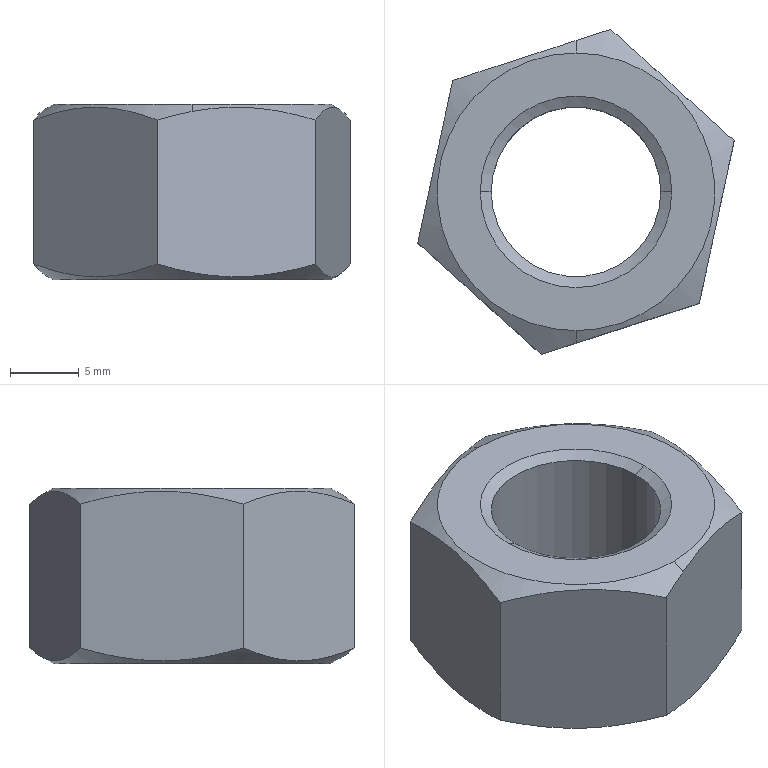Part | SolidWorks | features BaseBody 1 | 1 solid | 18 faces | box 23.075 x 23.71 x 12.8 mm | volume 3293 mm3 | cone 8 | plane 8 | cylinder 2 | commonest cylinder face diameters 12.376 x2
STEP:
#1=CARTESIAN_POINT('',(228.812,0.,355.481));
#2=VERTEX_POINT('',#1);
#3=CARTESIAN_POINT('',(241.188,0.,355.481));
#4=VERTEX_POINT('',#3);
#5=CARTESIAN_POINT('',(235.,0.,355.481));
#6=DIRECTION('',(0.,0.,1.));
#7=DIRECTION('',(1.,0.,0.));
#8=AXIS2_PLACEMENT_3D('',#5,#6,#7);
#9=CIRCLE('',#8,6.188);
#10=EDGE_CURVE('',#2,#4,#9,.T.);
#11=ORIENTED_EDGE('',*,*,#10,.F.);
#12=CARTESIAN_POINT('',(228.812,0.,367.019));
#13=VERTEX_POINT('',#12);
#14=CARTESIAN_POINT('',(228.812,0.,354.681));
#15=DIRECTION('',(0.,0.,1.));
#16=VECTOR('',#15,1000.);
#17=LINE('',#14,#16);
#18=EDGE_CURVE('',#2,#13,#17,.T.);
#19=ORIENTED_EDGE('',*,*,#18,.T.);
#20=CARTESIAN_POINT('',(241.188,0.,367.019));
#21=VERTEX_POINT('',#20);
#22=CARTESIAN_POINT('',(235.,0.,367.019));
#23=DIRECTION('',(0.,0.,-1.));
#24=DIRECTION('',(1.,0.,0.));
#25=AXIS2_PLACEMENT_3D('',#22,#23,#24);
#26=CIRCLE('',#25,6.188);
#27=EDGE_CURVE('',#21,#13,#26,.T.);
#28=ORIENTED_EDGE('',*,*,#27,.F.);
#29=CARTESIAN_POINT('',(241.188,0.,354.681));
#30=DIRECTION('',(0.,0.,1.));
#31=VECTOR('',#30,1000.);
#32=LINE('',#29,#31);
#33=EDGE_CURVE('',#4,#21,#32,.T.);
#34=ORIENTED_EDGE('',*,*,#33,.F.);
#35=EDGE_LOOP('',(#11,#19,#28,#34));
#36=FACE_OUTER_BOUND('',#35,.T.);
#37=CARTESIAN_POINT('',(235.,0.,354.681));
#38=DIRECTION('',(0.,0.,1.));
#39=DIRECTION('',(1.,0.,0.));
#40=AXIS2_PLACEMENT_3D('',#37,#38,#39);
#41=CYLINDRICAL_SURFACE('',#40,6.188);
#42=ADVANCED_FACE('',(#36),#41,.F.);
#43=ORIENTED_EDGE('',*,*,#27,.T.);
#44=CARTESIAN_POINT('',(228.012,0.,367.481));
#45=VERTEX_POINT('',#44);
#46=CARTESIAN_POINT('',(228.012,0.,367.481));
#47=DIRECTION('',(-0.866,0.,0.5));
#48=VECTOR('',#47,1000.);
#49=LINE('',#46,#48);
#50=EDGE_CURVE('',#13,#45,#49,.T.);
#51=ORIENTED_EDGE('',*,*,#50,.T.);
#52=CARTESIAN_POINT('',(241.988,0.,367.481));
#53=VERTEX_POINT('',#52);
#54=CARTESIAN_POINT('',(235.,0.,367.481));
#55=DIRECTION('',(0.,0.,-1.));
#56=DIRECTION('',(1.,0.,0.));
#57=AXIS2_PLACEMENT_3D('',#54,#55,#56);
#58=CIRCLE('',#57,6.988);
#59=EDGE_CURVE('',#53,#45,#58,.T.);
#60=ORIENTED_EDGE('',*,*,#59,.F.);
#61=CARTESIAN_POINT('',(241.988,0.,367.481));
#62=DIRECTION('',(0.866,0.,0.5));
#63=VECTOR('',#62,1000.);
#64=LINE('',#61,#63);
#65=EDGE_CURVE('',#21,#53,#64,.T.);
#66=ORIENTED_EDGE('',*,*,#65,.F.);
#67=EDGE_LOOP('',(#43,#51,#60,#66));
#68=FACE_OUTER_BOUND('',#67,.T.);
#69=CARTESIAN_POINT('',(235.,0.,367.481));
#70=DIRECTION('',(0.,0.,1.));
#71=DIRECTION('',(1.,0.,0.));
#72=AXIS2_PLACEMENT_3D('',#69,#70,#71);
#73=CONICAL_SURFACE('',#72,6.988,1.047);
#74=ADVANCED_FACE('',(#68),#73,.F.);
#75=ORIENTED_EDGE('',*,*,#10,.T.);
#76=CARTESIAN_POINT('',(241.65,0.,354.681));
#77=VERTEX_POINT('',#76);
#78=CARTESIAN_POINT('',(241.65,0.,354.681));
#79=DIRECTION('',(0.5,0.,-0.866));
#80=VECTOR('',#79,1000.);
#81=LINE('',#78,#80);
#82=EDGE_CURVE('',#4,#77,#81,.T.);
#83=ORIENTED_EDGE('',*,*,#82,.T.);
#84=CARTESIAN_POINT('',(228.35,0.,354.681));
#85=VERTEX_POINT('',#84);
#86=CARTESIAN_POINT('',(235.,0.,354.681));
#87=DIRECTION('',(0.,0.,1.));
#88=DIRECTION('',(-1.,0.,0.));
#89=AXIS2_PLACEMENT_3D('',#86,#87,#88);
#90=CIRCLE('',#89,6.65);
#91=EDGE_CURVE('',#85,#77,#90,.T.);
#92=ORIENTED_EDGE('',*,*,#91,.F.);
#93=CARTESIAN_POINT('',(228.35,0.,354.681));
#94=DIRECTION('',(-0.5,0.,-0.866));
#95=VECTOR('',#94,1000.);
#96=LINE('',#93,#95);
#97=EDGE_CURVE('',#2,#85,#96,.T.);
#98=ORIENTED_EDGE('',*,*,#97,.F.);
#99=EDGE_LOOP('',(#75,#83,#92,#98));
#100=FACE_OUTER_BOUND('',#99,.T.);
#101=CARTESIAN_POINT('',(235.,0.,354.681));
#102=DIRECTION('',(0.,0.,-1.));
#103=DIRECTION('',(-1.,0.,0.));
#104=AXIS2_PLACEMENT_3D('',#101,#102,#103);
#105=CONICAL_SURFACE('',#104,6.65,0.5236);
#106=ADVANCED_FACE('',(#100),#105,.F.);
#107=CARTESIAN_POINT('',(235.,-10.125,367.481));
#108=VERTEX_POINT('',#107);
#109=CARTESIAN_POINT('',(235.,10.125,367.481));
#110=VERTEX_POINT('',#109);
#111=CARTESIAN_POINT('',(235.,0.,367.481));
#112=DIRECTION('',(0.,0.,1.));
#113=DIRECTION('',(0.,1.,0.));
#114=AXIS2_PLACEMENT_3D('',#111,#112,#113);
#115=CIRCLE('',#114,10.125);
#116=EDGE_CURVE('',#108,#110,#115,.T.);
#117=ORIENTED_EDGE('',*,*,#116,.F.);
#118=CARTESIAN_POINT('',(235.,-11.034,366.956));
#119=VERTEX_POINT('',#118);
#120=CARTESIAN_POINT('',(235.,-12.136,366.32));
#121=DIRECTION('',(0.,-0.866,-0.5));
#122=VECTOR('',#121,1000.);
#123=LINE('',#120,#122);
#124=EDGE_CURVE('',#108,#119,#123,.T.);
#125=ORIENTED_EDGE('',*,*,#124,.T.);
#126=CARTESIAN_POINT('',(243.995,-8.129,366.327));
#127=VERTEX_POINT('',#126);
#128=CARTESIAN_POINT('',(235.,-11.034,366.956));
#129=CARTESIAN_POINT('',(235.743,-10.794,367.095));
#130=CARTESIAN_POINT('',(236.492,-10.552,367.191));
#131=CARTESIAN_POINT('',(237.626,-10.186,367.258));
#132=CARTESIAN_POINT('',(238.005,-10.063,367.267));
#133=CARTESIAN_POINT('',(238.768,-9.817,367.26));
#134=CARTESIAN_POINT('',(239.151,-9.694,367.243));
#135=CARTESIAN_POINT('',(241.046,-9.082,367.094));
#136=CARTESIAN_POINT('',(242.53,-8.602,366.771));
#137=CARTESIAN_POINT('',(243.995,-8.129,366.327));
#138=B_SPLINE_CURVE_WITH_KNOTS('',3,(#128,#129,#130,#131,#132,#133,#134,#135,#136,#137),.UNSPECIFIED.,.F.,.F.,(4,2,2,2,4),(0.002734,0.005112,0.006301,0.007489,0.01224),.UNSPECIFIED.);
#139=EDGE_CURVE('',#119,#127,#138,.T.);
#140=ORIENTED_EDGE('',*,*,#139,.T.);
#141=CARTESIAN_POINT('',(246.538,3.726,366.327));
#142=VERTEX_POINT('',#141);
#143=CARTESIAN_POINT('',(243.995,-8.129,366.327));
#144=CARTESIAN_POINT('',(244.203,-7.161,366.612));
#145=CARTESIAN_POINT('',(244.412,-6.186,366.848));
#146=CARTESIAN_POINT('',(244.835,-4.216,367.174));
#147=CARTESIAN_POINT('',(245.048,-3.221,367.264));
#148=CARTESIAN_POINT('',(245.372,-1.709,367.265));
#149=CARTESIAN_POINT('',(245.481,-1.203,367.243));
#150=CARTESIAN_POINT('',(245.696,-0.2013,367.157));
#151=CARTESIAN_POINT('',(245.802,0.2961,367.094));
#152=CARTESIAN_POINT('',(246.12,1.779,366.849));
#153=CARTESIAN_POINT('',(246.33,2.757,366.613));
#154=CARTESIAN_POINT('',(246.538,3.726,366.327));
#155=B_SPLINE_CURVE_WITH_KNOTS('',3,(#143,#144,#145,#146,#147,#148,#149,#150,#151,#152,#153,#154),.UNSPECIFIED.,.F.,.F.,(4,2,2,2,2,4),(0.,0.003061,0.006122,0.007653,0.009184,0.01224),.UNSPECIFIED.);
#156=EDGE_CURVE('',#127,#142,#155,.T.);
#157=ORIENTED_EDGE('',*,*,#156,.T.);
#158=CARTESIAN_POINT('',(237.542,11.855,366.327));
#159=VERTEX_POINT('',#158);
#160=CARTESIAN_POINT('',(246.538,3.726,366.327));
#161=CARTESIAN_POINT('',(245.803,4.39,366.613));
#162=CARTESIAN_POINT('',(245.062,5.059,366.848));
#163=CARTESIAN_POINT('',(243.565,6.412,367.175));
#164=CARTESIAN_POINT('',(242.808,7.097,367.265));
#165=CARTESIAN_POINT('',(241.272,8.484,367.265));
#166=CARTESIAN_POINT('',(240.515,9.168,367.175));
#167=CARTESIAN_POINT('',(239.018,10.522,366.848));
#168=CARTESIAN_POINT('',(238.277,11.191,366.613));
#169=CARTESIAN_POINT('',(237.542,11.855,366.327));
#170=B_SPLINE_CURVE_WITH_KNOTS('',3,(#160,#161,#162,#163,#164,#165,#166,#167,#168,#169),.UNSPECIFIED.,.F.,.F.,(4,2,2,2,4),(0.,0.003067,0.006134,0.009201,0.01227),.UNSPECIFIED.);
#171=EDGE_CURVE('',#142,#159,#170,.T.);
#172=ORIENTED_EDGE('',*,*,#171,.T.);
#173=CARTESIAN_POINT('',(235.,11.034,366.956));
#174=VERTEX_POINT('',#173);
#175=CARTESIAN_POINT('',(237.542,11.855,366.327));
#176=CARTESIAN_POINT('',(236.701,11.583,366.582));
#177=CARTESIAN_POINT('',(235.854,11.31,366.797));
#178=CARTESIAN_POINT('',(235.,11.034,366.956));
#179=B_SPLINE_CURVE_WITH_KNOTS('',3,(#175,#176,#177,#178),.UNSPECIFIED.,.F.,.F.,(4,4),(0.,0.002734),.UNSPECIFIED.);
#180=EDGE_CURVE('',#159,#174,#179,.T.);
#181=ORIENTED_EDGE('',*,*,#180,.T.);
#182=CARTESIAN_POINT('',(235.,12.136,366.32));
#183=DIRECTION('',(0.,0.866,-0.5));
#184=VECTOR('',#183,1000.);
#185=LINE('',#182,#184);
#186=EDGE_CURVE('',#110,#174,#185,.T.);
#187=ORIENTED_EDGE('',*,*,#186,.F.);
#188=EDGE_LOOP('',(#117,#125,#140,#157,#172,#181,#187));
#189=FACE_OUTER_BOUND('',#188,.T.);
#190=CARTESIAN_POINT('',(235.,0.,366.32));
#191=DIRECTION('',(0.,0.,-1.));
#192=DIRECTION('',(0.,1.,0.));
#193=AXIS2_PLACEMENT_3D('',#190,#191,#192);
#194=CONICAL_SURFACE('',#193,12.136,1.047);
#195=ADVANCED_FACE('',(#189),#194,.T.);
#196=CARTESIAN_POINT('',(245.125,0.,354.681));
#197=VERTEX_POINT('',#196);
#198=CARTESIAN_POINT('',(224.875,0.,354.681));
#199=VERTEX_POINT('',#198);
#200=CARTESIAN_POINT('',(235.,0.,354.681));
#201=DIRECTION('',(0.,0.,1.));
#202=DIRECTION('',(1.,0.,0.));
#203=AXIS2_PLACEMENT_3D('',#200,#201,#202);
#204=CIRCLE('',#203,10.125);
#205=EDGE_CURVE('',#197,#199,#204,.T.);
#206=ORIENTED_EDGE('',*,*,#205,.T.);
#207=CARTESIAN_POINT('',(224.261,0.,355.035));
#208=VERTEX_POINT('',#207);
#209=CARTESIAN_POINT('',(222.864,0.,355.842));
#210=DIRECTION('',(-0.866,0.,0.5));
#211=VECTOR('',#210,1000.);
#212=LINE('',#209,#211);
#213=EDGE_CURVE('',#199,#208,#212,.T.);
#214=ORIENTED_EDGE('',*,*,#213,.T.);
#215=CARTESIAN_POINT('',(226.005,8.129,355.835));
#216=VERTEX_POINT('',#215);
#217=CARTESIAN_POINT('',(224.261,0.,355.035));
#218=CARTESIAN_POINT('',(224.406,0.6764,354.952));
#219=CARTESIAN_POINT('',(224.552,1.358,354.904));
#220=CARTESIAN_POINT('',(224.774,2.389,354.895));
#221=CARTESIAN_POINT('',(224.848,2.735,354.902));
#222=CARTESIAN_POINT('',(224.995,3.422,354.937));
#223=CARTESIAN_POINT('',(225.069,3.765,354.964));
#224=CARTESIAN_POINT('',(225.434,5.468,355.148));
#225=CARTESIAN_POINT('',(225.721,6.806,355.445));
#226=CARTESIAN_POINT('',(226.005,8.129,355.835));
#227=B_SPLINE_CURVE_WITH_KNOTS('',3,(#217,#218,#219,#220,#221,#222,#223,#224,#225,#226),.UNSPECIFIED.,.F.,.F.,(4,2,2,2,4),(0.003885,0.005975,0.00702,0.008065,0.01224),.UNSPECIFIED.);
#228=EDGE_CURVE('',#208,#216,#227,.T.);
#229=ORIENTED_EDGE('',*,*,#228,.T.);
#230=CARTESIAN_POINT('',(237.542,11.855,355.835));
#231=VERTEX_POINT('',#230);
#232=CARTESIAN_POINT('',(226.005,8.129,355.835));
#233=CARTESIAN_POINT('',(226.947,8.433,355.55));
#234=CARTESIAN_POINT('',(227.895,8.74,355.314));
#235=CARTESIAN_POINT('',(229.813,9.359,354.988));
#236=CARTESIAN_POINT('',(230.782,9.672,354.898));
#237=CARTESIAN_POINT('',(232.253,10.147,354.897));
#238=CARTESIAN_POINT('',(232.746,10.306,354.919));
#239=CARTESIAN_POINT('',(233.72,10.621,355.005));
#240=CARTESIAN_POINT('',(234.205,10.777,355.068));
#241=CARTESIAN_POINT('',(235.648,11.243,355.313));
#242=CARTESIAN_POINT('',(236.599,11.55,355.549));
#243=CARTESIAN_POINT('',(237.542,11.855,355.835));
#244=B_SPLINE_CURVE_WITH_KNOTS('',3,(#232,#233,#234,#235,#236,#237,#238,#239,#240,#241,#242,#243),.UNSPECIFIED.,.F.,.F.,(4,2,2,2,2,4),(0.,0.003061,0.006122,0.007653,0.009184,0.01224),.UNSPECIFIED.);
#245=EDGE_CURVE('',#216,#231,#244,.T.);
#246=ORIENTED_EDGE('',*,*,#245,.T.);
#247=CARTESIAN_POINT('',(246.538,3.726,355.835));
#248=VERTEX_POINT('',#247);
#249=CARTESIAN_POINT('',(237.542,11.855,355.835));
#250=CARTESIAN_POINT('',(238.277,11.191,355.549));
#251=CARTESIAN_POINT('',(239.018,10.522,355.314));
#252=CARTESIAN_POINT('',(240.515,9.168,354.987));
#253=CARTESIAN_POINT('',(241.272,8.484,354.898));
#254=CARTESIAN_POINT('',(242.808,7.097,354.898));
#255=CARTESIAN_POINT('',(243.565,6.412,354.987));
#256=CARTESIAN_POINT('',(245.062,5.059,355.314));
#257=CARTESIAN_POINT('',(245.803,4.39,355.549));
#258=CARTESIAN_POINT('',(246.538,3.726,355.835));
#259=B_SPLINE_CURVE_WITH_KNOTS('',3,(#249,#250,#251,#252,#253,#254,#255,#256,#257,#258),.UNSPECIFIED.,.F.,.F.,(4,2,2,2,4),(-0.006134,-0.003067,0.,0.003067,0.006134),.UNSPECIFIED.);
#260=EDGE_CURVE('',#231,#248,#259,.T.);
#261=ORIENTED_EDGE('',*,*,#260,.T.);
#262=CARTESIAN_POINT('',(245.739,0.,355.035));
#263=VERTEX_POINT('',#262);
#264=CARTESIAN_POINT('',(246.538,3.726,355.835));
#265=CARTESIAN_POINT('',(246.274,2.497,355.473));
#266=CARTESIAN_POINT('',(246.008,1.257,355.191));
#267=CARTESIAN_POINT('',(245.739,0.,355.035));
#268=B_SPLINE_CURVE_WITH_KNOTS('',3,(#264,#265,#266,#267),.UNSPECIFIED.,.F.,.F.,(4,4),(0.,0.003885),.UNSPECIFIED.);
#269=EDGE_CURVE('',#248,#263,#268,.T.);
#270=ORIENTED_EDGE('',*,*,#269,.T.);
#271=CARTESIAN_POINT('',(247.136,0.,355.842));
#272=DIRECTION('',(0.866,0.,0.5));
#273=VECTOR('',#272,1000.);
#274=LINE('',#271,#273);
#275=EDGE_CURVE('',#197,#263,#274,.T.);
#276=ORIENTED_EDGE('',*,*,#275,.F.);
#277=EDGE_LOOP('',(#206,#214,#229,#246,#261,#270,#276));
#278=FACE_OUTER_BOUND('',#277,.T.);
#279=CARTESIAN_POINT('',(235.,0.,355.842));
#280=DIRECTION('',(0.,0.,1.));
#281=DIRECTION('',(1.,0.,0.));
#282=AXIS2_PLACEMENT_3D('',#279,#280,#281);
#283=CONICAL_SURFACE('',#282,12.136,1.047);
#284=ADVANCED_FACE('',(#278),#283,.T.);
#285=ORIENTED_EDGE('',*,*,#18,.F.);
#286=CARTESIAN_POINT('',(235.,0.,355.481));
#287=DIRECTION('',(0.,0.,1.));
#288=DIRECTION('',(1.,0.,0.));
#289=AXIS2_PLACEMENT_3D('',#286,#287,#288);
#290=CIRCLE('',#289,6.188);
#291=EDGE_CURVE('',#4,#2,#290,.T.);
#292=ORIENTED_EDGE('',*,*,#291,.F.);
#293=ORIENTED_EDGE('',*,*,#33,.T.);
#294=CARTESIAN_POINT('',(235.,0.,367.019));
#295=DIRECTION('',(0.,0.,-1.));
#296=DIRECTION('',(1.,0.,0.));
#297=AXIS2_PLACEMENT_3D('',#294,#295,#296);
#298=CIRCLE('',#297,6.188);
#299=EDGE_CURVE('',#13,#21,#298,.T.);
#300=ORIENTED_EDGE('',*,*,#299,.F.);
#301=EDGE_LOOP('',(#285,#292,#293,#300));
#302=FACE_OUTER_BOUND('',#301,.T.);
#303=CARTESIAN_POINT('',(235.,0.,354.681));
#304=DIRECTION('',(0.,0.,1.));
#305=DIRECTION('',(1.,0.,0.));
#306=AXIS2_PLACEMENT_3D('',#303,#304,#305);
#307=CYLINDRICAL_SURFACE('',#306,6.188);
#308=ADVANCED_FACE('',(#302),#307,.F.);
#309=ORIENTED_EDGE('',*,*,#50,.F.);
#310=ORIENTED_EDGE('',*,*,#299,.T.);
#311=ORIENTED_EDGE('',*,*,#65,.T.);
#312=CARTESIAN_POINT('',(235.,0.,367.481));
#313=DIRECTION('',(0.,0.,-1.));
#314=DIRECTION('',(1.,0.,0.));
#315=AXIS2_PLACEMENT_3D('',#312,#313,#314);
#316=CIRCLE('',#315,6.988);
#317=EDGE_CURVE('',#45,#53,#316,.T.);
#318=ORIENTED_EDGE('',*,*,#317,.F.);
#319=EDGE_LOOP('',(#309,#310,#311,#318));
#320=FACE_OUTER_BOUND('',#319,.T.);
#321=CARTESIAN_POINT('',(235.,0.,367.481));
#322=DIRECTION('',(0.,0.,1.));
#323=DIRECTION('',(1.,0.,0.));
#324=AXIS2_PLACEMENT_3D('',#321,#322,#323);
#325=CONICAL_SURFACE('',#324,6.988,1.047);
#326=ADVANCED_FACE('',(#320),#325,.F.);
#327=ORIENTED_EDGE('',*,*,#82,.F.);
#328=ORIENTED_EDGE('',*,*,#291,.T.);
#329=ORIENTED_EDGE('',*,*,#97,.T.);
#330=CARTESIAN_POINT('',(235.,0.,354.681));
#331=DIRECTION('',(0.,0.,1.));
#332=DIRECTION('',(-1.,0.,0.));
#333=AXIS2_PLACEMENT_3D('',#330,#331,#332);
#334=CIRCLE('',#333,6.65);
#335=EDGE_CURVE('',#77,#85,#334,.T.);
#336=ORIENTED_EDGE('',*,*,#335,.F.);
#337=EDGE_LOOP('',(#327,#328,#329,#336));
#338=FACE_OUTER_BOUND('',#337,.T.);
#339=CARTESIAN_POINT('',(235.,0.,354.681));
#340=DIRECTION('',(0.,0.,-1.));
#341=DIRECTION('',(-1.,0.,0.));
#342=AXIS2_PLACEMENT_3D('',#339,#340,#341);
#343=CONICAL_SURFACE('',#342,6.65,0.5236);
#344=ADVANCED_FACE('',(#338),#343,.F.);
#345=CARTESIAN_POINT('',(235.,0.,367.481));
#346=DIRECTION('',(0.,0.,1.));
#347=DIRECTION('',(0.,1.,0.));
#348=AXIS2_PLACEMENT_3D('',#345,#346,#347);
#349=CIRCLE('',#348,10.125);
#350=EDGE_CURVE('',#110,#108,#349,.T.);
#351=ORIENTED_EDGE('',*,*,#350,.T.);
#352=ORIENTED_EDGE('',*,*,#116,.T.);
#353=EDGE_LOOP('',(#351,#352));
#354=FACE_OUTER_BOUND('',#353,.T.);
#355=ORIENTED_EDGE('',*,*,#59,.T.);
#356=ORIENTED_EDGE('',*,*,#317,.T.);
#357=EDGE_LOOP('',(#355,#356));
#358=FACE_BOUND('',#357,.T.);
#359=CARTESIAN_POINT('',(228.547,19.984,367.481));
#360=DIRECTION('',(0.,0.,1.));
#361=DIRECTION('',(1.,0.,0.));
#362=AXIS2_PLACEMENT_3D('',#359,#360,#361);
#363=PLANE('',#362);
#364=ADVANCED_FACE('',(#354,#358),#363,.T.);
#365=ORIENTED_EDGE('',*,*,#205,.F.);
#366=CARTESIAN_POINT('',(235.,0.,354.681));
#367=DIRECTION('',(0.,0.,1.));
#368=DIRECTION('',(1.,0.,0.));
#369=AXIS2_PLACEMENT_3D('',#366,#367,#368);
#370=CIRCLE('',#369,10.125);
#371=EDGE_CURVE('',#199,#197,#370,.T.);
#372=ORIENTED_EDGE('',*,*,#371,.F.);
#373=EDGE_LOOP('',(#365,#372));
#374=FACE_OUTER_BOUND('',#373,.T.);
#375=ORIENTED_EDGE('',*,*,#91,.T.);
#376=ORIENTED_EDGE('',*,*,#335,.T.);
#377=EDGE_LOOP('',(#375,#376));
#378=FACE_BOUND('',#377,.T.);
#379=CARTESIAN_POINT('',(228.547,19.984,354.681));
#380=DIRECTION('',(0.,0.,1.));
#381=DIRECTION('',(1.,0.,0.));
#382=AXIS2_PLACEMENT_3D('',#379,#380,#381);
#383=PLANE('',#382);
#384=ADVANCED_FACE('',(#374,#378),#383,.F.);
#385=ORIENTED_EDGE('',*,*,#124,.F.);
#386=ORIENTED_EDGE('',*,*,#350,.F.);
#387=ORIENTED_EDGE('',*,*,#186,.T.);
#388=CARTESIAN_POINT('',(226.005,8.129,366.327));
#389=VERTEX_POINT('',#388);
#390=CARTESIAN_POINT('',(235.,11.034,366.956));
#391=CARTESIAN_POINT('',(234.257,10.794,367.095));
#392=CARTESIAN_POINT('',(233.508,10.552,367.191));
#393=CARTESIAN_POINT('',(232.374,10.186,367.258));
#394=CARTESIAN_POINT('',(231.995,10.063,367.267));
#395=CARTESIAN_POINT('',(231.232,9.817,367.26));
#396=CARTESIAN_POINT('',(230.849,9.694,367.243));
#397=CARTESIAN_POINT('',(228.954,9.082,367.094));
#398=CARTESIAN_POINT('',(227.47,8.602,366.771));
#399=CARTESIAN_POINT('',(226.005,8.129,366.327));
#400=B_SPLINE_CURVE_WITH_KNOTS('',3,(#390,#391,#392,#393,#394,#395,#396,#397,#398,#399),.UNSPECIFIED.,.F.,.F.,(4,2,2,2,4),(0.002734,0.005112,0.006301,0.007489,0.01224),.UNSPECIFIED.);
#401=EDGE_CURVE('',#174,#389,#400,.T.);
#402=ORIENTED_EDGE('',*,*,#401,.T.);
#403=CARTESIAN_POINT('',(223.462,-3.726,366.327));
#404=VERTEX_POINT('',#403);
#405=CARTESIAN_POINT('',(226.005,8.129,366.327));
#406=CARTESIAN_POINT('',(225.797,7.161,366.612));
#407=CARTESIAN_POINT('',(225.588,6.186,366.848));
#408=CARTESIAN_POINT('',(225.165,4.216,367.174));
#409=CARTESIAN_POINT('',(224.952,3.221,367.264));
#410=CARTESIAN_POINT('',(224.628,1.709,367.265));
#411=CARTESIAN_POINT('',(224.519,1.203,367.243));
#412=CARTESIAN_POINT('',(224.304,0.2013,367.157));
#413=CARTESIAN_POINT('',(224.198,-0.2961,367.094));
#414=CARTESIAN_POINT('',(223.88,-1.779,366.849));
#415=CARTESIAN_POINT('',(223.67,-2.757,366.613));
#416=CARTESIAN_POINT('',(223.462,-3.726,366.327));
#417=B_SPLINE_CURVE_WITH_KNOTS('',3,(#405,#406,#407,#408,#409,#410,#411,#412,#413,#414,#415,#416),.UNSPECIFIED.,.F.,.F.,(4,2,2,2,2,4),(0.,0.003061,0.006122,0.007653,0.009184,0.01224),.UNSPECIFIED.);
#418=EDGE_CURVE('',#389,#404,#417,.T.);
#419=ORIENTED_EDGE('',*,*,#418,.T.);
#420=CARTESIAN_POINT('',(232.458,-11.855,366.327));
#421=VERTEX_POINT('',#420);
#422=CARTESIAN_POINT('',(223.462,-3.726,366.327));
#423=CARTESIAN_POINT('',(224.197,-4.39,366.613));
#424=CARTESIAN_POINT('',(224.938,-5.059,366.848));
#425=CARTESIAN_POINT('',(226.435,-6.412,367.175));
#426=CARTESIAN_POINT('',(227.192,-7.097,367.265));
#427=CARTESIAN_POINT('',(228.728,-8.484,367.265));
#428=CARTESIAN_POINT('',(229.485,-9.168,367.175));
#429=CARTESIAN_POINT('',(230.982,-10.522,366.848));
#430=CARTESIAN_POINT('',(231.723,-11.191,366.613));
#431=CARTESIAN_POINT('',(232.458,-11.855,366.327));
#432=B_SPLINE_CURVE_WITH_KNOTS('',3,(#422,#423,#424,#425,#426,#427,#428,#429,#430,#431),.UNSPECIFIED.,.F.,.F.,(4,2,2,2,4),(-0.006134,-0.003067,0.,0.003067,0.006134),.UNSPECIFIED.);
#433=EDGE_CURVE('',#404,#421,#432,.T.);
#434=ORIENTED_EDGE('',*,*,#433,.T.);
#435=CARTESIAN_POINT('',(232.458,-11.855,366.327));
#436=CARTESIAN_POINT('',(233.299,-11.583,366.582));
#437=CARTESIAN_POINT('',(234.146,-11.31,366.797));
#438=CARTESIAN_POINT('',(235.,-11.034,366.956));
#439=B_SPLINE_CURVE_WITH_KNOTS('',3,(#435,#436,#437,#438),.UNSPECIFIED.,.F.,.F.,(4,4),(0.,0.002734),.UNSPECIFIED.);
#440=EDGE_CURVE('',#421,#119,#439,.T.);
#441=ORIENTED_EDGE('',*,*,#440,.T.);
#442=EDGE_LOOP('',(#385,#386,#387,#402,#419,#434,#441));
#443=FACE_OUTER_BOUND('',#442,.T.);
#444=CARTESIAN_POINT('',(235.,0.,366.32));
#445=DIRECTION('',(0.,0.,-1.));
#446=DIRECTION('',(0.,1.,0.));
#447=AXIS2_PLACEMENT_3D('',#444,#445,#446);
#448=CONICAL_SURFACE('',#447,12.136,1.047);
#449=ADVANCED_FACE('',(#443),#448,.T.);
#450=ORIENTED_EDGE('',*,*,#213,.F.);
#451=ORIENTED_EDGE('',*,*,#371,.T.);
#452=ORIENTED_EDGE('',*,*,#275,.T.);
#453=CARTESIAN_POINT('',(243.995,-8.129,355.835));
#454=VERTEX_POINT('',#453);
#455=CARTESIAN_POINT('',(245.739,0.,355.035));
#456=CARTESIAN_POINT('',(245.594,-0.6764,354.952));
#457=CARTESIAN_POINT('',(245.448,-1.358,354.904));
#458=CARTESIAN_POINT('',(245.226,-2.389,354.895));
#459=CARTESIAN_POINT('',(245.152,-2.735,354.902));
#460=CARTESIAN_POINT('',(245.005,-3.422,354.937));
#461=CARTESIAN_POINT('',(244.931,-3.765,354.964));
#462=CARTESIAN_POINT('',(244.566,-5.468,355.148));
#463=CARTESIAN_POINT('',(244.279,-6.806,355.445));
#464=CARTESIAN_POINT('',(243.995,-8.129,355.835));
#465=B_SPLINE_CURVE_WITH_KNOTS('',3,(#455,#456,#457,#458,#459,#460,#461,#462,#463,#464),.UNSPECIFIED.,.F.,.F.,(4,2,2,2,4),(0.003885,0.005975,0.00702,0.008065,0.01224),.UNSPECIFIED.);
#466=EDGE_CURVE('',#263,#454,#465,.T.);
#467=ORIENTED_EDGE('',*,*,#466,.T.);
#468=CARTESIAN_POINT('',(232.458,-11.855,355.835));
#469=VERTEX_POINT('',#468);
#470=CARTESIAN_POINT('',(243.995,-8.129,355.835));
#471=CARTESIAN_POINT('',(243.053,-8.433,355.55));
#472=CARTESIAN_POINT('',(242.105,-8.74,355.314));
#473=CARTESIAN_POINT('',(240.187,-9.359,354.988));
#474=CARTESIAN_POINT('',(239.218,-9.672,354.898));
#475=CARTESIAN_POINT('',(237.747,-10.147,354.897));
#476=CARTESIAN_POINT('',(237.254,-10.306,354.919));
#477=CARTESIAN_POINT('',(236.28,-10.621,355.005));
#478=CARTESIAN_POINT('',(235.795,-10.777,355.068));
#479=CARTESIAN_POINT('',(234.352,-11.243,355.313));
#480=CARTESIAN_POINT('',(233.401,-11.55,355.549));
#481=CARTESIAN_POINT('',(232.458,-11.855,355.835));
#482=B_SPLINE_CURVE_WITH_KNOTS('',3,(#470,#471,#472,#473,#474,#475,#476,#477,#478,#479,#480,#481),.UNSPECIFIED.,.F.,.F.,(4,2,2,2,2,4),(0.,0.003061,0.006122,0.007653,0.009184,0.01224),.UNSPECIFIED.);
#483=EDGE_CURVE('',#454,#469,#482,.T.);
#484=ORIENTED_EDGE('',*,*,#483,.T.);
#485=CARTESIAN_POINT('',(223.462,-3.726,355.835));
#486=VERTEX_POINT('',#485);
#487=CARTESIAN_POINT('',(232.458,-11.855,355.835));
#488=CARTESIAN_POINT('',(231.723,-11.191,355.549));
#489=CARTESIAN_POINT('',(230.982,-10.522,355.314));
#490=CARTESIAN_POINT('',(229.485,-9.168,354.987));
#491=CARTESIAN_POINT('',(228.728,-8.484,354.898));
#492=CARTESIAN_POINT('',(227.192,-7.097,354.898));
#493=CARTESIAN_POINT('',(226.435,-6.412,354.987));
#494=CARTESIAN_POINT('',(224.938,-5.059,355.314));
#495=CARTESIAN_POINT('',(224.197,-4.39,355.549));
#496=CARTESIAN_POINT('',(223.462,-3.726,355.835));
#497=B_SPLINE_CURVE_WITH_KNOTS('',3,(#487,#488,#489,#490,#491,#492,#493,#494,#495,#496),.UNSPECIFIED.,.F.,.F.,(4,2,2,2,4),(0.,0.003067,0.006134,0.009201,0.01227),.UNSPECIFIED.);
#498=EDGE_CURVE('',#469,#486,#497,.T.);
#499=ORIENTED_EDGE('',*,*,#498,.T.);
#500=CARTESIAN_POINT('',(223.462,-3.726,355.835));
#501=CARTESIAN_POINT('',(223.726,-2.497,355.473));
#502=CARTESIAN_POINT('',(223.992,-1.257,355.191));
#503=CARTESIAN_POINT('',(224.261,0.,355.035));
#504=B_SPLINE_CURVE_WITH_KNOTS('',3,(#500,#501,#502,#503),.UNSPECIFIED.,.F.,.F.,(4,4),(0.,0.003885),.UNSPECIFIED.);
#505=EDGE_CURVE('',#486,#208,#504,.T.);
#506=ORIENTED_EDGE('',*,*,#505,.T.);
#507=EDGE_LOOP('',(#450,#451,#452,#467,#484,#499,#506));
#508=FACE_OUTER_BOUND('',#507,.T.);
#509=CARTESIAN_POINT('',(235.,0.,355.842));
#510=DIRECTION('',(0.,0.,1.));
#511=DIRECTION('',(1.,0.,0.));
#512=AXIS2_PLACEMENT_3D('',#509,#510,#511);
#513=CONICAL_SURFACE('',#512,12.136,1.047);
#514=ADVANCED_FACE('',(#508),#513,.T.);
#515=ORIENTED_EDGE('',*,*,#260,.F.);
#516=CARTESIAN_POINT('',(237.542,11.855,354.681));
#517=DIRECTION('',(0.,0.,1.));
#518=VECTOR('',#517,1000.);
#519=LINE('',#516,#518);
#520=EDGE_CURVE('',#231,#159,#519,.T.);
#521=ORIENTED_EDGE('',*,*,#520,.T.);
#522=ORIENTED_EDGE('',*,*,#171,.F.);
#523=CARTESIAN_POINT('',(246.538,3.726,354.681));
#524=DIRECTION('',(0.,0.,-1.));
#525=VECTOR('',#524,1000.);
#526=LINE('',#523,#525);
#527=EDGE_CURVE('',#142,#248,#526,.T.);
#528=ORIENTED_EDGE('',*,*,#527,.T.);
#529=EDGE_LOOP('',(#515,#521,#522,#528));
#530=FACE_OUTER_BOUND('',#529,.T.);
#531=CARTESIAN_POINT('',(246.538,3.726,354.681));
#532=DIRECTION('',(0.6705,0.7419,0.));
#533=DIRECTION('',(-0.7419,0.6705,0.));
#534=AXIS2_PLACEMENT_3D('',#531,#532,#533);
#535=PLANE('',#534);
#536=ADVANCED_FACE('',(#530),#535,.T.);
#537=ORIENTED_EDGE('',*,*,#269,.F.);
#538=ORIENTED_EDGE('',*,*,#527,.F.);
#539=ORIENTED_EDGE('',*,*,#156,.F.);
#540=CARTESIAN_POINT('',(243.995,-8.129,354.681));
#541=DIRECTION('',(0.,0.,-1.));
#542=VECTOR('',#541,1000.);
#543=LINE('',#540,#542);
#544=EDGE_CURVE('',#127,#454,#543,.T.);
#545=ORIENTED_EDGE('',*,*,#544,.T.);
#546=ORIENTED_EDGE('',*,*,#466,.F.);
#547=EDGE_LOOP('',(#537,#538,#539,#545,#546));
#548=FACE_OUTER_BOUND('',#547,.T.);
#549=CARTESIAN_POINT('',(243.995,-8.129,354.681));
#550=DIRECTION('',(0.9778,-0.2097,0.));
#551=DIRECTION('',(0.2097,0.9778,0.));
#552=AXIS2_PLACEMENT_3D('',#549,#550,#551);
#553=PLANE('',#552);
#554=ADVANCED_FACE('',(#548),#553,.T.);
#555=ORIENTED_EDGE('',*,*,#483,.F.);
#556=ORIENTED_EDGE('',*,*,#544,.F.);
#557=ORIENTED_EDGE('',*,*,#139,.F.);
#558=ORIENTED_EDGE('',*,*,#440,.F.);
#559=CARTESIAN_POINT('',(232.458,-11.855,354.681));
#560=DIRECTION('',(0.,0.,-1.));
#561=VECTOR('',#560,1000.);
#562=LINE('',#559,#561);
#563=EDGE_CURVE('',#421,#469,#562,.T.);
#564=ORIENTED_EDGE('',*,*,#563,.T.);
#565=EDGE_LOOP('',(#555,#556,#557,#558,#564));
#566=FACE_OUTER_BOUND('',#565,.T.);
#567=CARTESIAN_POINT('',(232.458,-11.855,354.681));
#568=DIRECTION('',(0.3073,-0.9516,0.));
#569=DIRECTION('',(0.9516,0.3073,0.));
#570=AXIS2_PLACEMENT_3D('',#567,#568,#569);
#571=PLANE('',#570);
#572=ADVANCED_FACE('',(#566),#571,.T.);
#573=ORIENTED_EDGE('',*,*,#498,.F.);
#574=ORIENTED_EDGE('',*,*,#563,.F.);
#575=ORIENTED_EDGE('',*,*,#433,.F.);
#576=CARTESIAN_POINT('',(223.462,-3.726,354.681));
#577=DIRECTION('',(0.,0.,-1.));
#578=VECTOR('',#577,1000.);
#579=LINE('',#576,#578);
#580=EDGE_CURVE('',#404,#486,#579,.T.);
#581=ORIENTED_EDGE('',*,*,#580,.T.);
#582=EDGE_LOOP('',(#573,#574,#575,#581));
#583=FACE_OUTER_BOUND('',#582,.T.);
#584=CARTESIAN_POINT('',(223.462,-3.726,354.681));
#585=DIRECTION('',(-0.6705,-0.7419,0.));
#586=DIRECTION('',(0.7419,-0.6705,0.));
#587=AXIS2_PLACEMENT_3D('',#584,#585,#586);
#588=PLANE('',#587);
#589=ADVANCED_FACE('',(#583),#588,.T.);
#590=ORIENTED_EDGE('',*,*,#505,.F.);
#591=ORIENTED_EDGE('',*,*,#580,.F.);
#592=ORIENTED_EDGE('',*,*,#418,.F.);
#593=CARTESIAN_POINT('',(226.005,8.129,354.681));
#594=DIRECTION('',(0.,0.,-1.));
#595=VECTOR('',#594,1000.);
#596=LINE('',#593,#595);
#597=EDGE_CURVE('',#389,#216,#596,.T.);
#598=ORIENTED_EDGE('',*,*,#597,.T.);
#599=ORIENTED_EDGE('',*,*,#228,.F.);
#600=EDGE_LOOP('',(#590,#591,#592,#598,#599));
#601=FACE_OUTER_BOUND('',#600,.T.);
#602=CARTESIAN_POINT('',(226.005,8.129,354.681));
#603=DIRECTION('',(-0.9778,0.2097,0.));
#604=DIRECTION('',(-0.2097,-0.9778,0.));
#605=AXIS2_PLACEMENT_3D('',#602,#603,#604);
#606=PLANE('',#605);
#607=ADVANCED_FACE('',(#601),#606,.T.);
#608=ORIENTED_EDGE('',*,*,#245,.F.);
#609=ORIENTED_EDGE('',*,*,#597,.F.);
#610=ORIENTED_EDGE('',*,*,#401,.F.);
#611=ORIENTED_EDGE('',*,*,#180,.F.);
#612=ORIENTED_EDGE('',*,*,#520,.F.);
#613=EDGE_LOOP('',(#608,#609,#610,#611,#612));
#614=FACE_OUTER_BOUND('',#613,.T.);
#615=CARTESIAN_POINT('',(237.542,11.855,354.681));
#616=DIRECTION('',(-0.3073,0.9516,0.));
#617=DIRECTION('',(-0.9516,-0.3073,0.));
#618=AXIS2_PLACEMENT_3D('',#615,#616,#617);
#619=PLANE('',#618);
#620=ADVANCED_FACE('',(#614),#619,.T.);
#621=CLOSED_SHELL('',(#42,#74,#106,#195,#284,#308,#326,#344,#364,#384,#449,#514,#536,#554,#572,#589,#607,#620));
#622=MANIFOLD_SOLID_BREP('',#621);
#623=CARTESIAN_POINT('',(0.,0.,0.));
#624=DIRECTION('',(0.,0.,1.));
#625=DIRECTION('',(1.,0.,0.));
#626=AXIS2_PLACEMENT_3D('',#623,#624,#625);
#627=(LENGTH_UNIT()NAMED_UNIT(*)SI_UNIT(.MILLI.,.METRE.));
#628=UNCERTAINTY_MEASURE_WITH_UNIT(LENGTH_MEASURE(0.00001),#627,'','');
#629=(NAMED_UNIT(*)PLANE_ANGLE_UNIT()SI_UNIT($,.RADIAN.));
#630=(NAMED_UNIT(*)SI_UNIT($,.STERADIAN.)SOLID_ANGLE_UNIT());
#631=(GEOMETRIC_REPRESENTATION_CONTEXT(3)GLOBAL_UNCERTAINTY_ASSIGNED_CONTEXT((#628))GLOBAL_UNIT_ASSIGNED_CONTEXT((#627,#629,#630))REPRESENTATION_CONTEXT('',''));
#632=ADVANCED_BREP_SHAPE_REPRESENTATION('',(#622,#626),#631);